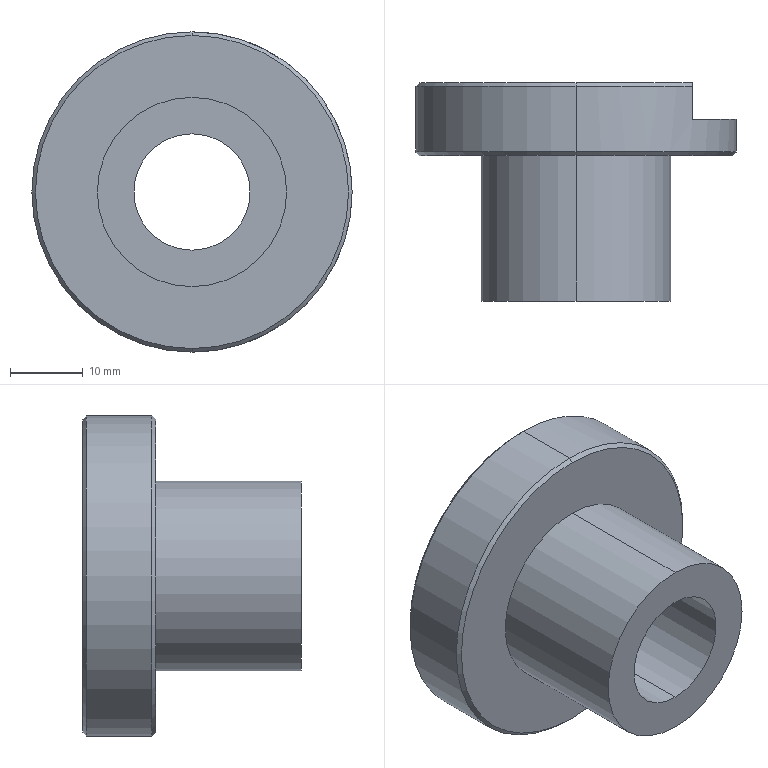Part | SolidWorks | features Chamfer 2, ICE 1, Revolution 1 | 1 solid | 18 faces | box 44 x 30 x 44 mm | volume 19113 mm3 | cone 7 | cylinder 6 | plane 5 | commonest cylinder face diameters 16 x2 26 x2 44 x2
STEP:
#1=CARTESIAN_POINT('',(0.,17.532,-8.));
#2=VERTEX_POINT('',#1);
#3=CARTESIAN_POINT('',(0.,17.532,8.));
#4=VERTEX_POINT('',#3);
#5=CARTESIAN_POINT('',(0.,17.532,0.));
#6=DIRECTION('',(0.,1.,0.));
#7=DIRECTION('',(0.,0.,1.));
#8=AXIS2_PLACEMENT_3D('',#5,#6,#7);
#9=CIRCLE('',#8,8.);
#10=EDGE_CURVE('',#2,#4,#9,.T.);
#11=ORIENTED_EDGE('',*,*,#10,.F.);
#12=CARTESIAN_POINT('',(0.,18.532,-9.));
#13=VERTEX_POINT('',#12);
#14=CARTESIAN_POINT('',(0.,17.532,-8.));
#15=DIRECTION('',(0.,0.7071,-0.7071));
#16=VECTOR('',#15,1000.);
#17=LINE('',#14,#16);
#18=EDGE_CURVE('',#2,#13,#17,.T.);
#19=ORIENTED_EDGE('',*,*,#18,.T.);
#20=CARTESIAN_POINT('',(0.,18.532,9.));
#21=VERTEX_POINT('',#20);
#22=CARTESIAN_POINT('',(0.,18.532,0.));
#23=DIRECTION('',(0.,-1.,0.));
#24=DIRECTION('',(0.,0.,1.));
#25=AXIS2_PLACEMENT_3D('',#22,#23,#24);
#26=CIRCLE('',#25,9.);
#27=EDGE_CURVE('',#21,#13,#26,.T.);
#28=ORIENTED_EDGE('',*,*,#27,.F.);
#29=CARTESIAN_POINT('',(0.,17.532,8.));
#30=DIRECTION('',(0.,0.7071,0.7071));
#31=VECTOR('',#30,1000.);
#32=LINE('',#29,#31);
#33=EDGE_CURVE('',#4,#21,#32,.T.);
#34=ORIENTED_EDGE('',*,*,#33,.F.);
#35=EDGE_LOOP('',(#11,#19,#28,#34));
#36=FACE_OUTER_BOUND('',#35,.T.);
#37=CARTESIAN_POINT('',(0.,17.532,0.));
#38=DIRECTION('',(0.,1.,0.));
#39=DIRECTION('',(0.,0.,1.));
#40=AXIS2_PLACEMENT_3D('',#37,#38,#39);
#41=CONICAL_SURFACE('',#40,8.,0.7854);
#42=ADVANCED_FACE('',(#36),#41,.F.);
#43=CARTESIAN_POINT('',(0.,18.532,21.5));
#44=VERTEX_POINT('',#43);
#45=CARTESIAN_POINT('',(16.,18.532,14.361));
#46=VERTEX_POINT('',#45);
#47=CARTESIAN_POINT('',(0.,18.532,0.));
#48=DIRECTION('',(0.,1.,0.));
#49=DIRECTION('',(0.,0.,1.));
#50=AXIS2_PLACEMENT_3D('',#47,#48,#49);
#51=CIRCLE('',#50,21.5);
#52=EDGE_CURVE('',#44,#46,#51,.T.);
#53=ORIENTED_EDGE('',*,*,#52,.F.);
#54=CARTESIAN_POINT('',(0.,18.032,22.));
#55=VERTEX_POINT('',#54);
#56=CARTESIAN_POINT('',(0.,18.532,21.5));
#57=DIRECTION('',(0.,-0.7071,0.7071));
#58=VECTOR('',#57,1000.);
#59=LINE('',#56,#58);
#60=EDGE_CURVE('',#44,#55,#59,.T.);
#61=ORIENTED_EDGE('',*,*,#60,.T.);
#62=CARTESIAN_POINT('',(16.,18.032,15.1));
#63=VERTEX_POINT('',#62);
#64=CARTESIAN_POINT('',(0.,18.032,0.));
#65=DIRECTION('',(0.,-1.,0.));
#66=DIRECTION('',(0.,0.,1.));
#67=AXIS2_PLACEMENT_3D('',#64,#65,#66);
#68=CIRCLE('',#67,22.);
#69=EDGE_CURVE('',#63,#55,#68,.T.);
#70=ORIENTED_EDGE('',*,*,#69,.F.);
#71=CARTESIAN_POINT('',(16.,18.532,14.361));
#72=CARTESIAN_POINT('',(16.,18.367,14.609));
#73=CARTESIAN_POINT('',(16.,18.2,14.855));
#74=CARTESIAN_POINT('',(16.,18.032,15.1));
#75=B_SPLINE_CURVE_WITH_KNOTS('',3,(#71,#72,#73,#74),.UNSPECIFIED.,.F.,.F.,(4,4),(0.07228,0.07316),.UNSPECIFIED.);
#76=EDGE_CURVE('',#46,#63,#75,.T.);
#77=ORIENTED_EDGE('',*,*,#76,.F.);
#78=EDGE_LOOP('',(#53,#61,#70,#77));
#79=FACE_OUTER_BOUND('',#78,.T.);
#80=CARTESIAN_POINT('',(0.,18.532,0.));
#81=DIRECTION('',(0.,-1.,0.));
#82=DIRECTION('',(0.,0.,-1.));
#83=AXIS2_PLACEMENT_3D('',#80,#81,#82);
#84=CONICAL_SURFACE('',#83,21.5,0.7854);
#85=ADVANCED_FACE('',(#79),#84,.T.);
#86=ORIENTED_EDGE('',*,*,#60,.F.);
#87=CARTESIAN_POINT('',(0.,18.532,-21.5));
#88=VERTEX_POINT('',#87);
#89=CARTESIAN_POINT('',(0.,18.532,0.));
#90=DIRECTION('',(0.,1.,0.));
#91=DIRECTION('',(0.,0.,1.));
#92=AXIS2_PLACEMENT_3D('',#89,#90,#91);
#93=CIRCLE('',#92,21.5);
#94=EDGE_CURVE('',#88,#44,#93,.T.);
#95=ORIENTED_EDGE('',*,*,#94,.F.);
#96=CARTESIAN_POINT('',(0.,18.032,-22.));
#97=VERTEX_POINT('',#96);
#98=CARTESIAN_POINT('',(0.,18.532,-21.5));
#99=DIRECTION('',(0.,-0.7071,-0.7071));
#100=VECTOR('',#99,1000.);
#101=LINE('',#98,#100);
#102=EDGE_CURVE('',#88,#97,#101,.T.);
#103=ORIENTED_EDGE('',*,*,#102,.T.);
#104=CARTESIAN_POINT('',(0.,18.032,0.));
#105=DIRECTION('',(0.,-1.,0.));
#106=DIRECTION('',(0.,0.,1.));
#107=AXIS2_PLACEMENT_3D('',#104,#105,#106);
#108=CIRCLE('',#107,22.);
#109=EDGE_CURVE('',#55,#97,#108,.T.);
#110=ORIENTED_EDGE('',*,*,#109,.F.);
#111=EDGE_LOOP('',(#86,#95,#103,#110));
#112=FACE_OUTER_BOUND('',#111,.T.);
#113=CARTESIAN_POINT('',(0.,18.532,0.));
#114=DIRECTION('',(0.,-1.,0.));
#115=DIRECTION('',(0.,0.,-1.));
#116=AXIS2_PLACEMENT_3D('',#113,#114,#115);
#117=CONICAL_SURFACE('',#116,21.5,0.7854);
#118=ADVANCED_FACE('',(#112),#117,.T.);
#119=CARTESIAN_POINT('',(0.,8.532,-21.5));
#120=VERTEX_POINT('',#119);
#121=CARTESIAN_POINT('',(0.,8.532,21.5));
#122=VERTEX_POINT('',#121);
#123=CARTESIAN_POINT('',(0.,8.532,0.));
#124=DIRECTION('',(0.,-1.,0.));
#125=DIRECTION('',(0.,0.,-1.));
#126=AXIS2_PLACEMENT_3D('',#123,#124,#125);
#127=CIRCLE('',#126,21.5);
#128=EDGE_CURVE('',#120,#122,#127,.T.);
#129=ORIENTED_EDGE('',*,*,#128,.F.);
#130=CARTESIAN_POINT('',(0.,9.032,-22.));
#131=VERTEX_POINT('',#130);
#132=CARTESIAN_POINT('',(0.,9.032,-22.));
#133=DIRECTION('',(0.,0.7071,-0.7071));
#134=VECTOR('',#133,1000.);
#135=LINE('',#132,#134);
#136=EDGE_CURVE('',#120,#131,#135,.T.);
#137=ORIENTED_EDGE('',*,*,#136,.T.);
#138=CARTESIAN_POINT('',(0.,9.032,22.));
#139=VERTEX_POINT('',#138);
#140=CARTESIAN_POINT('',(0.,9.032,0.));
#141=DIRECTION('',(0.,1.,0.));
#142=DIRECTION('',(0.,0.,-1.));
#143=AXIS2_PLACEMENT_3D('',#140,#141,#142);
#144=CIRCLE('',#143,22.);
#145=EDGE_CURVE('',#139,#131,#144,.T.);
#146=ORIENTED_EDGE('',*,*,#145,.F.);
#147=CARTESIAN_POINT('',(0.,9.032,22.));
#148=DIRECTION('',(0.,0.7071,0.7071));
#149=VECTOR('',#148,1000.);
#150=LINE('',#147,#149);
#151=EDGE_CURVE('',#122,#139,#150,.T.);
#152=ORIENTED_EDGE('',*,*,#151,.F.);
#153=EDGE_LOOP('',(#129,#137,#146,#152));
#154=FACE_OUTER_BOUND('',#153,.T.);
#155=CARTESIAN_POINT('',(0.,9.032,0.));
#156=DIRECTION('',(0.,1.,0.));
#157=DIRECTION('',(0.,0.,1.));
#158=AXIS2_PLACEMENT_3D('',#155,#156,#157);
#159=CONICAL_SURFACE('',#158,22.,0.7854);
#160=ADVANCED_FACE('',(#154),#159,.T.);
#161=CARTESIAN_POINT('',(0.,-11.468,-8.));
#162=VERTEX_POINT('',#161);
#163=CARTESIAN_POINT('',(0.,-11.468,8.));
#164=VERTEX_POINT('',#163);
#165=CARTESIAN_POINT('',(0.,-11.468,0.));
#166=DIRECTION('',(0.,1.,0.));
#167=DIRECTION('',(0.,0.,1.));
#168=AXIS2_PLACEMENT_3D('',#165,#166,#167);
#169=CIRCLE('',#168,8.);
#170=EDGE_CURVE('',#162,#164,#169,.T.);
#171=ORIENTED_EDGE('',*,*,#170,.F.);
#172=CARTESIAN_POINT('',(0.,40.811,-8.));
#173=DIRECTION('',(0.,1.,0.));
#174=VECTOR('',#173,1000.);
#175=LINE('',#172,#174);
#176=EDGE_CURVE('',#162,#2,#175,.T.);
#177=ORIENTED_EDGE('',*,*,#176,.T.);
#178=ORIENTED_EDGE('',*,*,#10,.T.);
#179=CARTESIAN_POINT('',(0.,40.811,8.));
#180=DIRECTION('',(0.,1.,0.));
#181=VECTOR('',#180,1000.);
#182=LINE('',#179,#181);
#183=EDGE_CURVE('',#164,#4,#182,.T.);
#184=ORIENTED_EDGE('',*,*,#183,.F.);
#185=EDGE_LOOP('',(#171,#177,#178,#184));
#186=FACE_OUTER_BOUND('',#185,.T.);
#187=CARTESIAN_POINT('',(0.,40.811,0.));
#188=DIRECTION('',(0.,1.,0.));
#189=DIRECTION('',(0.,0.,1.));
#190=AXIS2_PLACEMENT_3D('',#187,#188,#189);
#191=CYLINDRICAL_SURFACE('',#190,8.);
#192=ADVANCED_FACE('',(#186),#191,.F.);
#193=CARTESIAN_POINT('',(0.,-11.468,13.));
#194=VERTEX_POINT('',#193);
#195=CARTESIAN_POINT('',(0.,-11.468,-13.));
#196=VERTEX_POINT('',#195);
#197=CARTESIAN_POINT('',(0.,-11.468,0.));
#198=DIRECTION('',(0.,1.,0.));
#199=DIRECTION('',(0.,0.,1.));
#200=AXIS2_PLACEMENT_3D('',#197,#198,#199);
#201=CIRCLE('',#200,13.);
#202=EDGE_CURVE('',#194,#196,#201,.T.);
#203=ORIENTED_EDGE('',*,*,#202,.T.);
#204=CARTESIAN_POINT('',(0.,8.532,-13.));
#205=VERTEX_POINT('',#204);
#206=CARTESIAN_POINT('',(0.,40.811,-13.));
#207=DIRECTION('',(0.,1.,0.));
#208=VECTOR('',#207,1000.);
#209=LINE('',#206,#208);
#210=EDGE_CURVE('',#196,#205,#209,.T.);
#211=ORIENTED_EDGE('',*,*,#210,.T.);
#212=CARTESIAN_POINT('',(0.,8.532,13.));
#213=VERTEX_POINT('',#212);
#214=CARTESIAN_POINT('',(0.,8.532,0.));
#215=DIRECTION('',(0.,1.,0.));
#216=DIRECTION('',(0.,0.,1.));
#217=AXIS2_PLACEMENT_3D('',#214,#215,#216);
#218=CIRCLE('',#217,13.);
#219=EDGE_CURVE('',#213,#205,#218,.T.);
#220=ORIENTED_EDGE('',*,*,#219,.F.);
#221=CARTESIAN_POINT('',(0.,40.811,13.));
#222=DIRECTION('',(0.,1.,0.));
#223=VECTOR('',#222,1000.);
#224=LINE('',#221,#223);
#225=EDGE_CURVE('',#194,#213,#224,.T.);
#226=ORIENTED_EDGE('',*,*,#225,.F.);
#227=EDGE_LOOP('',(#203,#211,#220,#226));
#228=FACE_OUTER_BOUND('',#227,.T.);
#229=CARTESIAN_POINT('',(0.,40.811,0.));
#230=DIRECTION('',(0.,1.,0.));
#231=DIRECTION('',(0.,0.,1.));
#232=AXIS2_PLACEMENT_3D('',#229,#230,#231);
#233=CYLINDRICAL_SURFACE('',#232,13.);
#234=ADVANCED_FACE('',(#228),#233,.T.);
#235=ORIENTED_EDGE('',*,*,#145,.T.);
#236=CARTESIAN_POINT('',(0.,40.811,-22.));
#237=DIRECTION('',(0.,1.,0.));
#238=VECTOR('',#237,1000.);
#239=LINE('',#236,#238);
#240=EDGE_CURVE('',#131,#97,#239,.T.);
#241=ORIENTED_EDGE('',*,*,#240,.T.);
#242=CARTESIAN_POINT('',(16.,18.032,-15.1));
#243=VERTEX_POINT('',#242);
#244=CARTESIAN_POINT('',(0.,18.032,0.));
#245=DIRECTION('',(0.,-1.,0.));
#246=DIRECTION('',(0.,0.,1.));
#247=AXIS2_PLACEMENT_3D('',#244,#245,#246);
#248=CIRCLE('',#247,22.);
#249=EDGE_CURVE('',#97,#243,#248,.T.);
#250=ORIENTED_EDGE('',*,*,#249,.T.);
#251=CARTESIAN_POINT('',(16.,13.532,-15.1));
#252=VERTEX_POINT('',#251);
#253=CARTESIAN_POINT('',(16.,40.811,-15.1));
#254=DIRECTION('',(0.,1.,0.));
#255=VECTOR('',#254,1000.);
#256=LINE('',#253,#255);
#257=EDGE_CURVE('',#252,#243,#256,.T.);
#258=ORIENTED_EDGE('',*,*,#257,.F.);
#259=CARTESIAN_POINT('',(16.,13.532,15.1));
#260=VERTEX_POINT('',#259);
#261=CARTESIAN_POINT('',(0.,13.532,0.));
#262=DIRECTION('',(0.,-1.,0.));
#263=DIRECTION('',(0.,0.,1.));
#264=AXIS2_PLACEMENT_3D('',#261,#262,#263);
#265=CIRCLE('',#264,22.);
#266=EDGE_CURVE('',#252,#260,#265,.T.);
#267=ORIENTED_EDGE('',*,*,#266,.T.);
#268=CARTESIAN_POINT('',(16.,40.811,15.1));
#269=DIRECTION('',(0.,-1.,0.));
#270=VECTOR('',#269,1000.);
#271=LINE('',#268,#270);
#272=EDGE_CURVE('',#63,#260,#271,.T.);
#273=ORIENTED_EDGE('',*,*,#272,.F.);
#274=ORIENTED_EDGE('',*,*,#69,.T.);
#275=CARTESIAN_POINT('',(0.,40.811,22.));
#276=DIRECTION('',(0.,1.,0.));
#277=VECTOR('',#276,1000.);
#278=LINE('',#275,#277);
#279=EDGE_CURVE('',#139,#55,#278,.T.);
#280=ORIENTED_EDGE('',*,*,#279,.F.);
#281=EDGE_LOOP('',(#235,#241,#250,#258,#267,#273,#274,#280));
#282=FACE_OUTER_BOUND('',#281,.T.);
#283=CARTESIAN_POINT('',(0.,40.811,0.));
#284=DIRECTION('',(0.,1.,0.));
#285=DIRECTION('',(0.,0.,1.));
#286=AXIS2_PLACEMENT_3D('',#283,#284,#285);
#287=CYLINDRICAL_SURFACE('',#286,22.);
#288=ADVANCED_FACE('',(#282),#287,.T.);
#289=CARTESIAN_POINT('',(16.,18.532,-14.361));
#290=VERTEX_POINT('',#289);
#291=CARTESIAN_POINT('',(16.,18.532,-25.017));
#292=DIRECTION('',(0.,0.,1.));
#293=VECTOR('',#292,1000.);
#294=LINE('',#291,#293);
#295=EDGE_CURVE('',#290,#46,#294,.T.);
#296=ORIENTED_EDGE('',*,*,#295,.F.);
#297=CARTESIAN_POINT('',(0.,18.532,0.));
#298=DIRECTION('',(0.,1.,0.));
#299=DIRECTION('',(0.,0.,1.));
#300=AXIS2_PLACEMENT_3D('',#297,#298,#299);
#301=CIRCLE('',#300,21.5);
#302=EDGE_CURVE('',#290,#88,#301,.T.);
#303=ORIENTED_EDGE('',*,*,#302,.T.);
#304=ORIENTED_EDGE('',*,*,#94,.T.);
#305=ORIENTED_EDGE('',*,*,#52,.T.);
#306=EDGE_LOOP('',(#296,#303,#304,#305));
#307=FACE_OUTER_BOUND('',#306,.T.);
#308=ORIENTED_EDGE('',*,*,#27,.T.);
#309=CARTESIAN_POINT('',(0.,18.532,0.));
#310=DIRECTION('',(0.,-1.,0.));
#311=DIRECTION('',(0.,0.,1.));
#312=AXIS2_PLACEMENT_3D('',#309,#310,#311);
#313=CIRCLE('',#312,9.);
#314=EDGE_CURVE('',#13,#21,#313,.T.);
#315=ORIENTED_EDGE('',*,*,#314,.T.);
#316=EDGE_LOOP('',(#308,#315));
#317=FACE_BOUND('',#316,.T.);
#318=CARTESIAN_POINT('',(-8.,18.532,0.));
#319=DIRECTION('',(0.,1.,0.));
#320=DIRECTION('',(0.,0.,1.));
#321=AXIS2_PLACEMENT_3D('',#318,#319,#320);
#322=PLANE('',#321);
#323=ADVANCED_FACE('',(#307,#317),#322,.T.);
#324=ORIENTED_EDGE('',*,*,#240,.F.);
#325=CARTESIAN_POINT('',(0.,9.032,0.));
#326=DIRECTION('',(0.,1.,0.));
#327=DIRECTION('',(0.,0.,-1.));
#328=AXIS2_PLACEMENT_3D('',#325,#326,#327);
#329=CIRCLE('',#328,22.);
#330=EDGE_CURVE('',#131,#139,#329,.T.);
#331=ORIENTED_EDGE('',*,*,#330,.T.);
#332=ORIENTED_EDGE('',*,*,#279,.T.);
#333=ORIENTED_EDGE('',*,*,#109,.T.);
#334=EDGE_LOOP('',(#324,#331,#332,#333));
#335=FACE_OUTER_BOUND('',#334,.T.);
#336=CARTESIAN_POINT('',(0.,40.811,0.));
#337=DIRECTION('',(0.,1.,0.));
#338=DIRECTION('',(0.,0.,1.));
#339=AXIS2_PLACEMENT_3D('',#336,#337,#338);
#340=CYLINDRICAL_SURFACE('',#339,22.);
#341=ADVANCED_FACE('',(#335),#340,.T.);
#342=CARTESIAN_POINT('',(0.,8.532,0.));
#343=DIRECTION('',(0.,-1.,0.));
#344=DIRECTION('',(0.,0.,-1.));
#345=AXIS2_PLACEMENT_3D('',#342,#343,#344);
#346=CIRCLE('',#345,21.5);
#347=EDGE_CURVE('',#122,#120,#346,.T.);
#348=ORIENTED_EDGE('',*,*,#347,.T.);
#349=ORIENTED_EDGE('',*,*,#128,.T.);
#350=EDGE_LOOP('',(#348,#349));
#351=FACE_OUTER_BOUND('',#350,.T.);
#352=ORIENTED_EDGE('',*,*,#219,.T.);
#353=CARTESIAN_POINT('',(0.,8.532,0.));
#354=DIRECTION('',(0.,1.,0.));
#355=DIRECTION('',(0.,0.,1.));
#356=AXIS2_PLACEMENT_3D('',#353,#354,#355);
#357=CIRCLE('',#356,13.);
#358=EDGE_CURVE('',#205,#213,#357,.T.);
#359=ORIENTED_EDGE('',*,*,#358,.T.);
#360=EDGE_LOOP('',(#352,#359));
#361=FACE_BOUND('',#360,.T.);
#362=CARTESIAN_POINT('',(-22.,8.532,0.));
#363=DIRECTION('',(0.,-1.,0.));
#364=DIRECTION('',(0.,0.,-1.));
#365=AXIS2_PLACEMENT_3D('',#362,#363,#364);
#366=PLANE('',#365);
#367=ADVANCED_FACE('',(#351,#361),#366,.T.);
#368=ORIENTED_EDGE('',*,*,#210,.F.);
#369=CARTESIAN_POINT('',(0.,-11.468,0.));
#370=DIRECTION('',(0.,1.,0.));
#371=DIRECTION('',(0.,0.,1.));
#372=AXIS2_PLACEMENT_3D('',#369,#370,#371);
#373=CIRCLE('',#372,13.);
#374=EDGE_CURVE('',#196,#194,#373,.T.);
#375=ORIENTED_EDGE('',*,*,#374,.T.);
#376=ORIENTED_EDGE('',*,*,#225,.T.);
#377=ORIENTED_EDGE('',*,*,#358,.F.);
#378=EDGE_LOOP('',(#368,#375,#376,#377));
#379=FACE_OUTER_BOUND('',#378,.T.);
#380=CARTESIAN_POINT('',(0.,40.811,0.));
#381=DIRECTION('',(0.,1.,0.));
#382=DIRECTION('',(0.,0.,1.));
#383=AXIS2_PLACEMENT_3D('',#380,#381,#382);
#384=CYLINDRICAL_SURFACE('',#383,13.);
#385=ADVANCED_FACE('',(#379),#384,.T.);
#386=CARTESIAN_POINT('',(0.,-11.468,0.));
#387=DIRECTION('',(0.,1.,0.));
#388=DIRECTION('',(0.,0.,1.));
#389=AXIS2_PLACEMENT_3D('',#386,#387,#388);
#390=CIRCLE('',#389,8.);
#391=EDGE_CURVE('',#164,#162,#390,.T.);
#392=ORIENTED_EDGE('',*,*,#391,.T.);
#393=ORIENTED_EDGE('',*,*,#170,.T.);
#394=EDGE_LOOP('',(#392,#393));
#395=FACE_BOUND('',#394,.T.);
#396=ORIENTED_EDGE('',*,*,#202,.F.);
#397=ORIENTED_EDGE('',*,*,#374,.F.);
#398=EDGE_LOOP('',(#396,#397));
#399=FACE_OUTER_BOUND('',#398,.T.);
#400=CARTESIAN_POINT('',(-13.,-11.468,0.));
#401=DIRECTION('',(0.,-1.,0.));
#402=DIRECTION('',(0.,0.,-1.));
#403=AXIS2_PLACEMENT_3D('',#400,#401,#402);
#404=PLANE('',#403);
#405=ADVANCED_FACE('',(#395,#399),#404,.T.);
#406=ORIENTED_EDGE('',*,*,#176,.F.);
#407=ORIENTED_EDGE('',*,*,#391,.F.);
#408=ORIENTED_EDGE('',*,*,#183,.T.);
#409=CARTESIAN_POINT('',(0.,17.532,0.));
#410=DIRECTION('',(0.,1.,0.));
#411=DIRECTION('',(0.,0.,1.));
#412=AXIS2_PLACEMENT_3D('',#409,#410,#411);
#413=CIRCLE('',#412,8.);
#414=EDGE_CURVE('',#4,#2,#413,.T.);
#415=ORIENTED_EDGE('',*,*,#414,.T.);
#416=EDGE_LOOP('',(#406,#407,#408,#415));
#417=FACE_OUTER_BOUND('',#416,.T.);
#418=CARTESIAN_POINT('',(0.,40.811,0.));
#419=DIRECTION('',(0.,1.,0.));
#420=DIRECTION('',(0.,0.,1.));
#421=AXIS2_PLACEMENT_3D('',#418,#419,#420);
#422=CYLINDRICAL_SURFACE('',#421,8.);
#423=ADVANCED_FACE('',(#417),#422,.F.);
#424=ORIENTED_EDGE('',*,*,#136,.F.);
#425=ORIENTED_EDGE('',*,*,#347,.F.);
#426=ORIENTED_EDGE('',*,*,#151,.T.);
#427=ORIENTED_EDGE('',*,*,#330,.F.);
#428=EDGE_LOOP('',(#424,#425,#426,#427));
#429=FACE_OUTER_BOUND('',#428,.T.);
#430=CARTESIAN_POINT('',(0.,9.032,0.));
#431=DIRECTION('',(0.,1.,0.));
#432=DIRECTION('',(0.,0.,1.));
#433=AXIS2_PLACEMENT_3D('',#430,#431,#432);
#434=CONICAL_SURFACE('',#433,22.,0.7854);
#435=ADVANCED_FACE('',(#429),#434,.T.);
#436=ORIENTED_EDGE('',*,*,#102,.F.);
#437=ORIENTED_EDGE('',*,*,#302,.F.);
#438=CARTESIAN_POINT('',(16.,18.032,-15.1));
#439=CARTESIAN_POINT('',(16.,18.2,-14.855));
#440=CARTESIAN_POINT('',(16.,18.367,-14.609));
#441=CARTESIAN_POINT('',(16.,18.532,-14.361));
#442=B_SPLINE_CURVE_WITH_KNOTS('',3,(#438,#439,#440,#441),.UNSPECIFIED.,.F.,.F.,(4,4),(0.04047,0.04137),.UNSPECIFIED.);
#443=EDGE_CURVE('',#243,#290,#442,.T.);
#444=ORIENTED_EDGE('',*,*,#443,.F.);
#445=ORIENTED_EDGE('',*,*,#249,.F.);
#446=EDGE_LOOP('',(#436,#437,#444,#445));
#447=FACE_OUTER_BOUND('',#446,.T.);
#448=CARTESIAN_POINT('',(0.,18.532,0.));
#449=DIRECTION('',(0.,-1.,0.));
#450=DIRECTION('',(0.,0.,-1.));
#451=AXIS2_PLACEMENT_3D('',#448,#449,#450);
#452=CONICAL_SURFACE('',#451,21.5,0.7854);
#453=ADVANCED_FACE('',(#447),#452,.T.);
#454=ORIENTED_EDGE('',*,*,#18,.F.);
#455=ORIENTED_EDGE('',*,*,#414,.F.);
#456=ORIENTED_EDGE('',*,*,#33,.T.);
#457=ORIENTED_EDGE('',*,*,#314,.F.);
#458=EDGE_LOOP('',(#454,#455,#456,#457));
#459=FACE_OUTER_BOUND('',#458,.T.);
#460=CARTESIAN_POINT('',(0.,17.532,0.));
#461=DIRECTION('',(0.,1.,0.));
#462=DIRECTION('',(0.,0.,1.));
#463=AXIS2_PLACEMENT_3D('',#460,#461,#462);
#464=CONICAL_SURFACE('',#463,8.,0.7854);
#465=ADVANCED_FACE('',(#459),#464,.F.);
#466=ORIENTED_EDGE('',*,*,#257,.T.);
#467=ORIENTED_EDGE('',*,*,#443,.T.);
#468=ORIENTED_EDGE('',*,*,#295,.T.);
#469=ORIENTED_EDGE('',*,*,#76,.T.);
#470=ORIENTED_EDGE('',*,*,#272,.T.);
#471=CARTESIAN_POINT('',(16.,13.532,-25.017));
#472=DIRECTION('',(0.,0.,1.));
#473=VECTOR('',#472,1000.);
#474=LINE('',#471,#473);
#475=EDGE_CURVE('',#252,#260,#474,.T.);
#476=ORIENTED_EDGE('',*,*,#475,.F.);
#477=EDGE_LOOP('',(#466,#467,#468,#469,#470,#476));
#478=FACE_OUTER_BOUND('',#477,.T.);
#479=CARTESIAN_POINT('',(16.,13.532,-25.017));
#480=DIRECTION('',(-1.,0.,0.));
#481=DIRECTION('',(0.,0.,1.));
#482=AXIS2_PLACEMENT_3D('',#479,#480,#481);
#483=PLANE('',#482);
#484=ADVANCED_FACE('',(#478),#483,.F.);
#485=ORIENTED_EDGE('',*,*,#475,.T.);
#486=ORIENTED_EDGE('',*,*,#266,.F.);
#487=EDGE_LOOP('',(#485,#486));
#488=FACE_OUTER_BOUND('',#487,.T.);
#489=CARTESIAN_POINT('',(0.,13.532,0.));
#490=DIRECTION('',(0.,1.,0.));
#491=DIRECTION('',(0.,0.,1.));
#492=AXIS2_PLACEMENT_3D('',#489,#490,#491);
#493=PLANE('',#492);
#494=ADVANCED_FACE('',(#488),#493,.T.);
#495=CLOSED_SHELL('',(#42,#85,#118,#160,#192,#234,#288,#323,#341,#367,#385,#405,#423,#435,#453,#465,#484,#494));
#496=MANIFOLD_SOLID_BREP('',#495);
#497=CARTESIAN_POINT('',(0.,0.,0.));
#498=DIRECTION('',(0.,0.,1.));
#499=DIRECTION('',(1.,0.,0.));
#500=AXIS2_PLACEMENT_3D('',#497,#498,#499);
#501=(LENGTH_UNIT()NAMED_UNIT(*)SI_UNIT(.MILLI.,.METRE.));
#502=UNCERTAINTY_MEASURE_WITH_UNIT(LENGTH_MEASURE(0.00001),#501,'','');
#503=(NAMED_UNIT(*)PLANE_ANGLE_UNIT()SI_UNIT($,.RADIAN.));
#504=(NAMED_UNIT(*)SI_UNIT($,.STERADIAN.)SOLID_ANGLE_UNIT());
#505=(GEOMETRIC_REPRESENTATION_CONTEXT(3)GLOBAL_UNCERTAINTY_ASSIGNED_CONTEXT((#502))GLOBAL_UNIT_ASSIGNED_CONTEXT((#501,#503,#504))REPRESENTATION_CONTEXT('',''));
#506=ADVANCED_BREP_SHAPE_REPRESENTATION('',(#496,#500),#505);